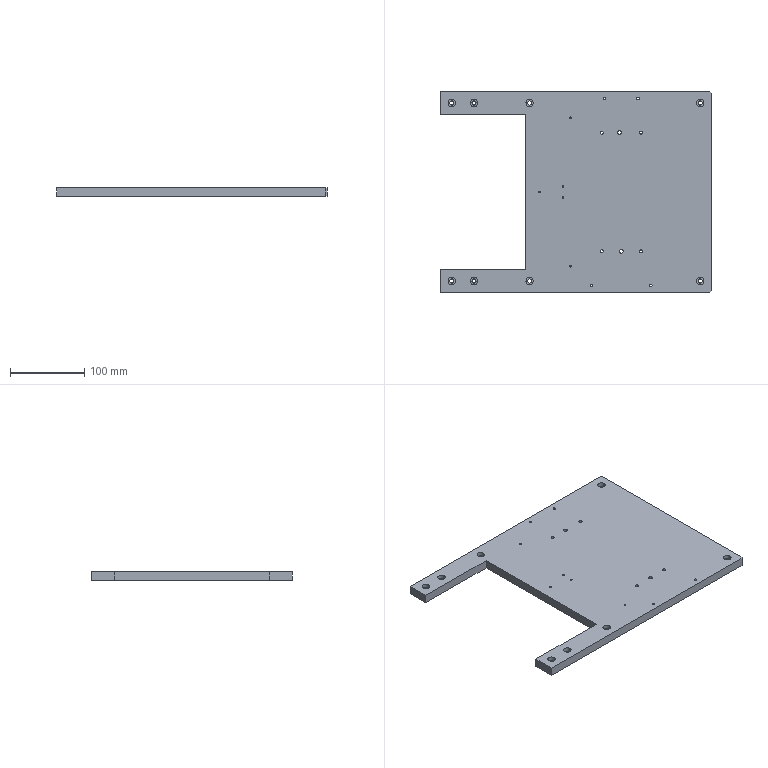Part | 1 solid | 96 faces | box 365 x 270 x 12 mm | volume 886330 mm3 | cylinder 64 | plane 20 | cone 12 | commonest cylinder face diameters 5.5 x16 10 x16 2.5 x12 3.3 x8 4.2 x8 5 x4